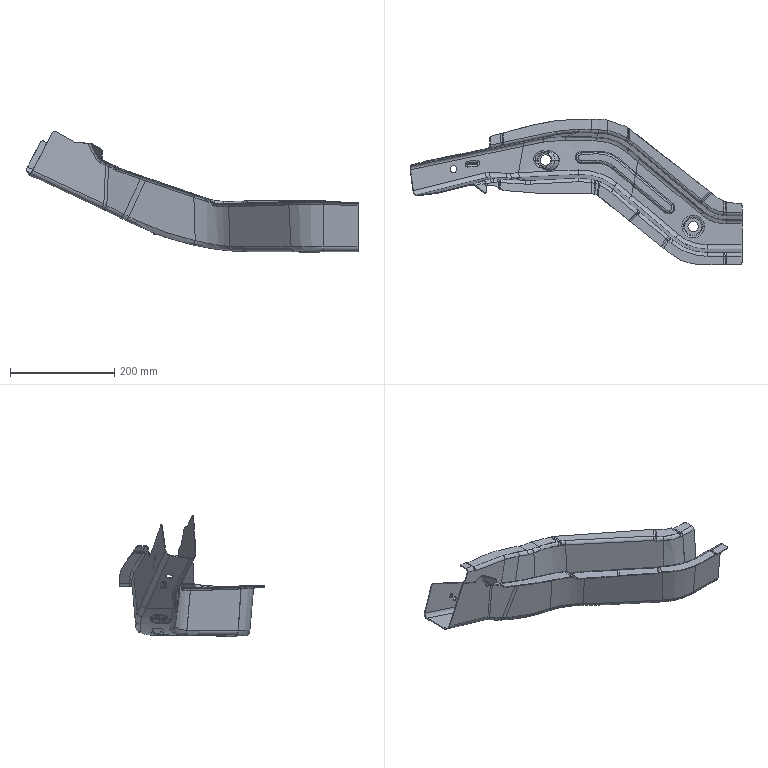Part | 1 solid | 494 faces | box 636.452 x 279.348 x 232.624 mm | volume 286381 mm3 | spline 301 | cylinder 128 | plane 49 | sphere 14 | other 2 | commonest cylinder face diameters 10 x28 13 x20 20 x12 8 x8 17 x8 7 x6